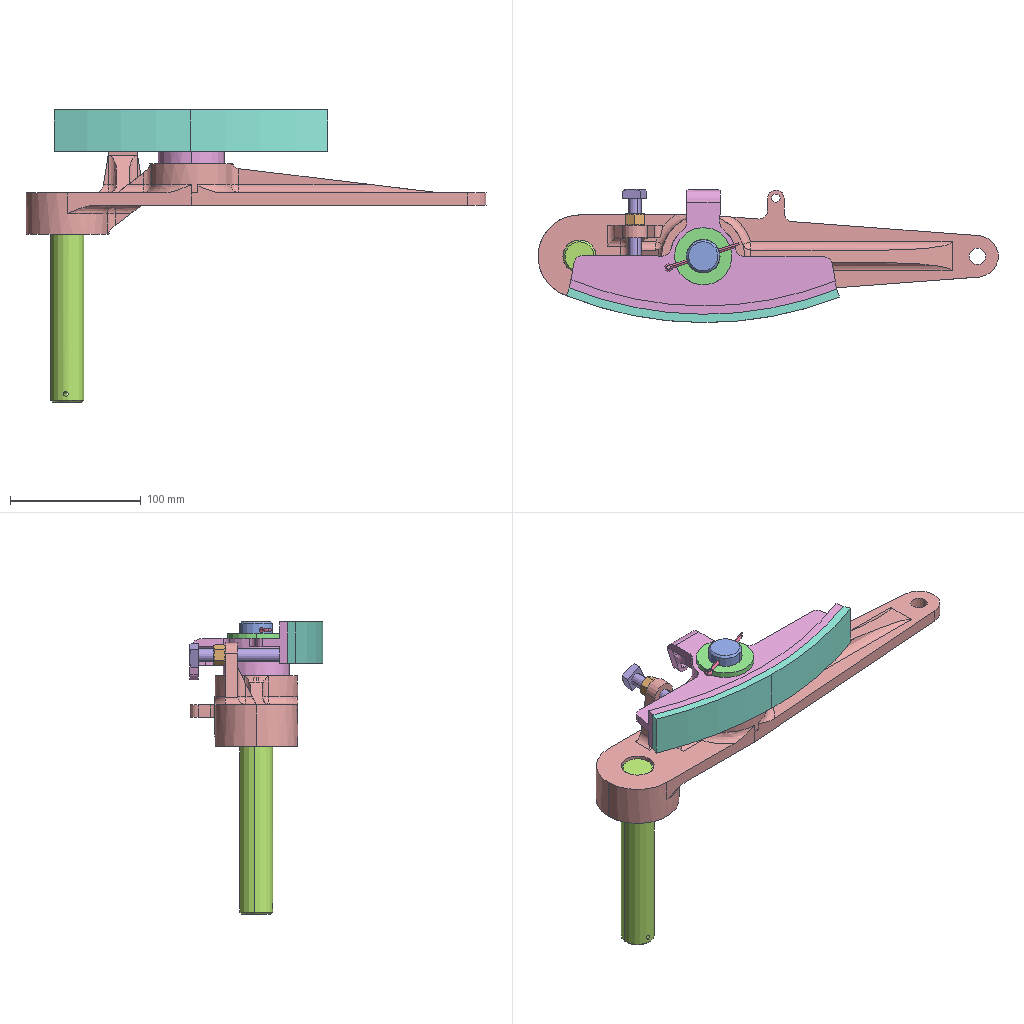Assembly | SolidWorks | 9 different items | 9 placed | box 352 x 102 x 224 mm
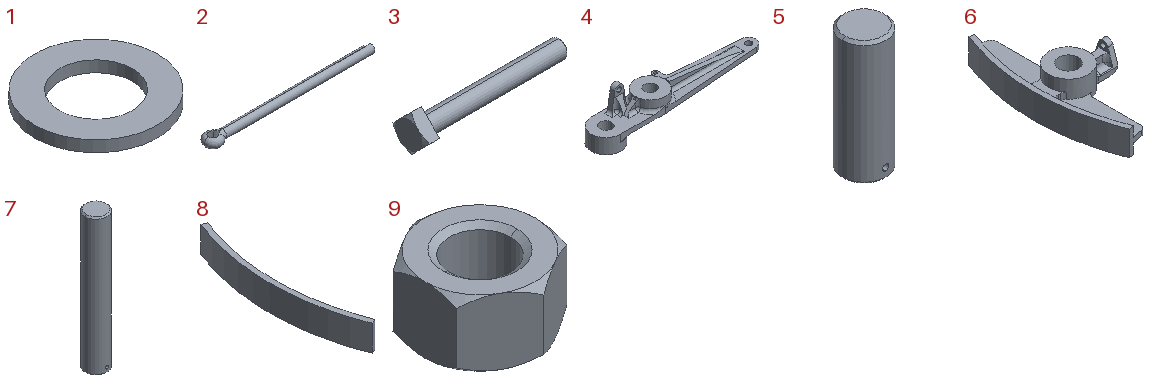Parts list (item | quantity | size | volume | features):
1 | x1 | 44 x 44 x 4 mm | 3958 mm3 | features Extrusion 1
2 | x1 | 186.3 x 19 x 9.5 mm | 13160 mm3 | features Sweep 1
3 | x1 | 83.007 x 20.188 x 20.188 mm | 6786 mm3 | features RevCut 2, Extrusion 1, Fillet 1, LPattern 1, Revolution 1
4 | x1 | 352.42 x 82.55 x 79.56 mm | 319205 mm3 | features Fillet 9, ICE 4, Rib 4, Extrusion 1
5 | x1 | 25.4 x 25.4 x 71.37 mm | 35732 mm3 | features Chamfer 1, Extrusion 1, ICE 1
6 | x1 | 95.24 x 204.62 x 44.45 mm | 132567 mm3 | features Fillet 7, ICE 6, Extrusion 1, Rib 1
7 | x1 | 25.4 x 25.4 x 158.75 mm | 80008 mm3 | features Chamfer 1, Extrusion 1, ICE 1
8 | x1 | 25.986 x 209.322 x 31.75 mm | 42745 mm3 | features Extrusion 1
9 | x1 | 14.275 x 16.483 x 8.56 mm | 1065 mm3 | features RevCut 4, Extrusion 1, LPattern 1
Mates (type | each side: item.copy, entity, surface, feature):
Concentric | 4.1 face cylinder Cut-Extrude1 | 5.1 face cylinder Boss-Extrude1
DistanceDim | 5.1 face plane Boss-Extrude1 | 4.1 face plane Boss-Extrude3
Concentric | 4.1 face cylinder Boss-Extrude1 | 7.1 face cylinder Boss-Extrude1
DistanceDim | 7.1 face plane Boss-Extrude1 | 4.1 face plane Boss-Extrude2
Coincident | 4.1 face plane Boss-Extrude3 | 6.1 face plane Boss-Extrude3
Concentric | 5.1 face cylinder Boss-Extrude1 | 6.1 face cylinder Cut-Extrude2
Concentric | 6.1 face cylinder Boss-Extrude1 | 8.1 face cylinder Boss-Extrude1
Coincident | 6.1 edge | 8.1 edge
Coincident | 6.1 face plane Boss-Extrude1 | 8.1 face plane Boss-Extrude1
Concentric | 4.1 face cylinder Boss-Extrude4 | 9.1 face cylinder EndChamfer
Coincident | 4.1 face plane Boss-Extrude4 | 9.1 face plane BaseNut
Concentric | 9.1 face cylinder BaseNut | 3.1 face cylinder Body
Concentric | 6.1 face cylinder Cut-Extrude2 | 1.1 face cylinder Base-Extrude
Coincident | 6.1 face plane Boss-Extrude2 | 1.1 face plane Base-Extrude
Concentric | 5.1 face cylinder Cut-Extrude1 | 2.1 face cylinder Body
DistanceDim | 2.1 face plane Body | 5.1 plane